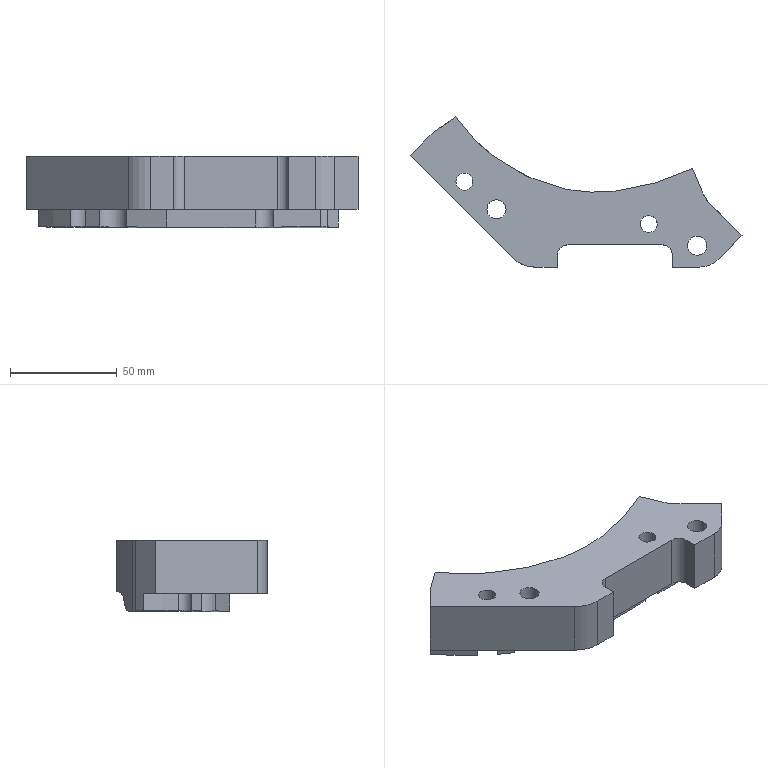Part | STEP file | 814_id1586_x_t | 1 solid | 62 faces | box 155.471 x 70.307 x 33.716 mm | volume 123664 mm3 | spline 26 | plane 21 | cylinder 15 | commonest cylinder face diameters 10 x5 30 x3 8 x2 9 x2 14 x2 24 x1